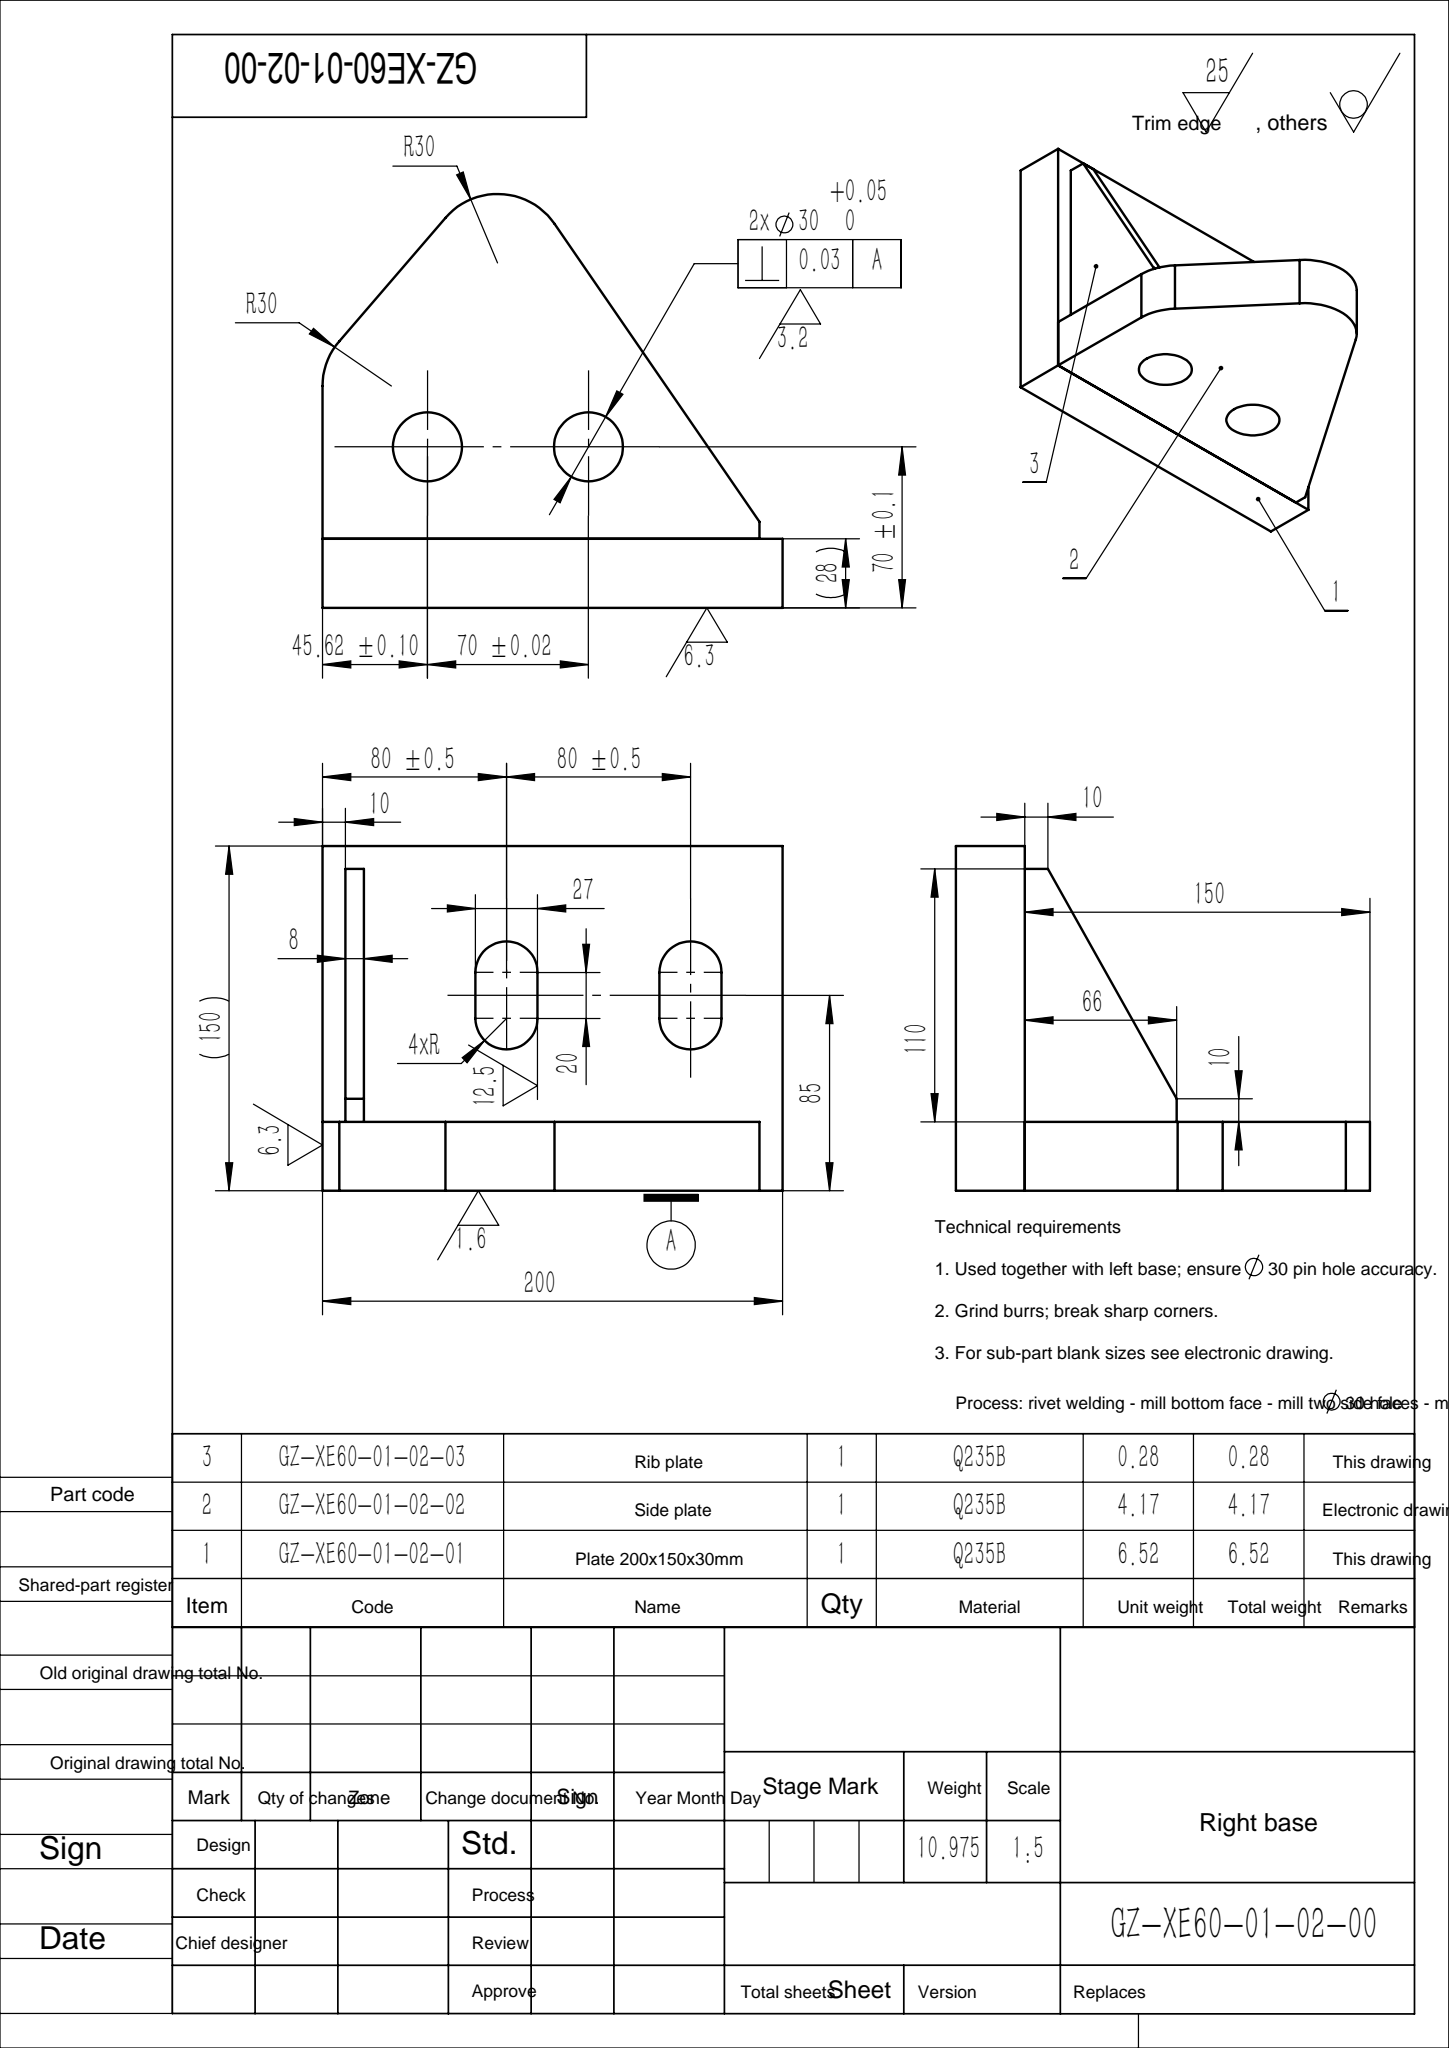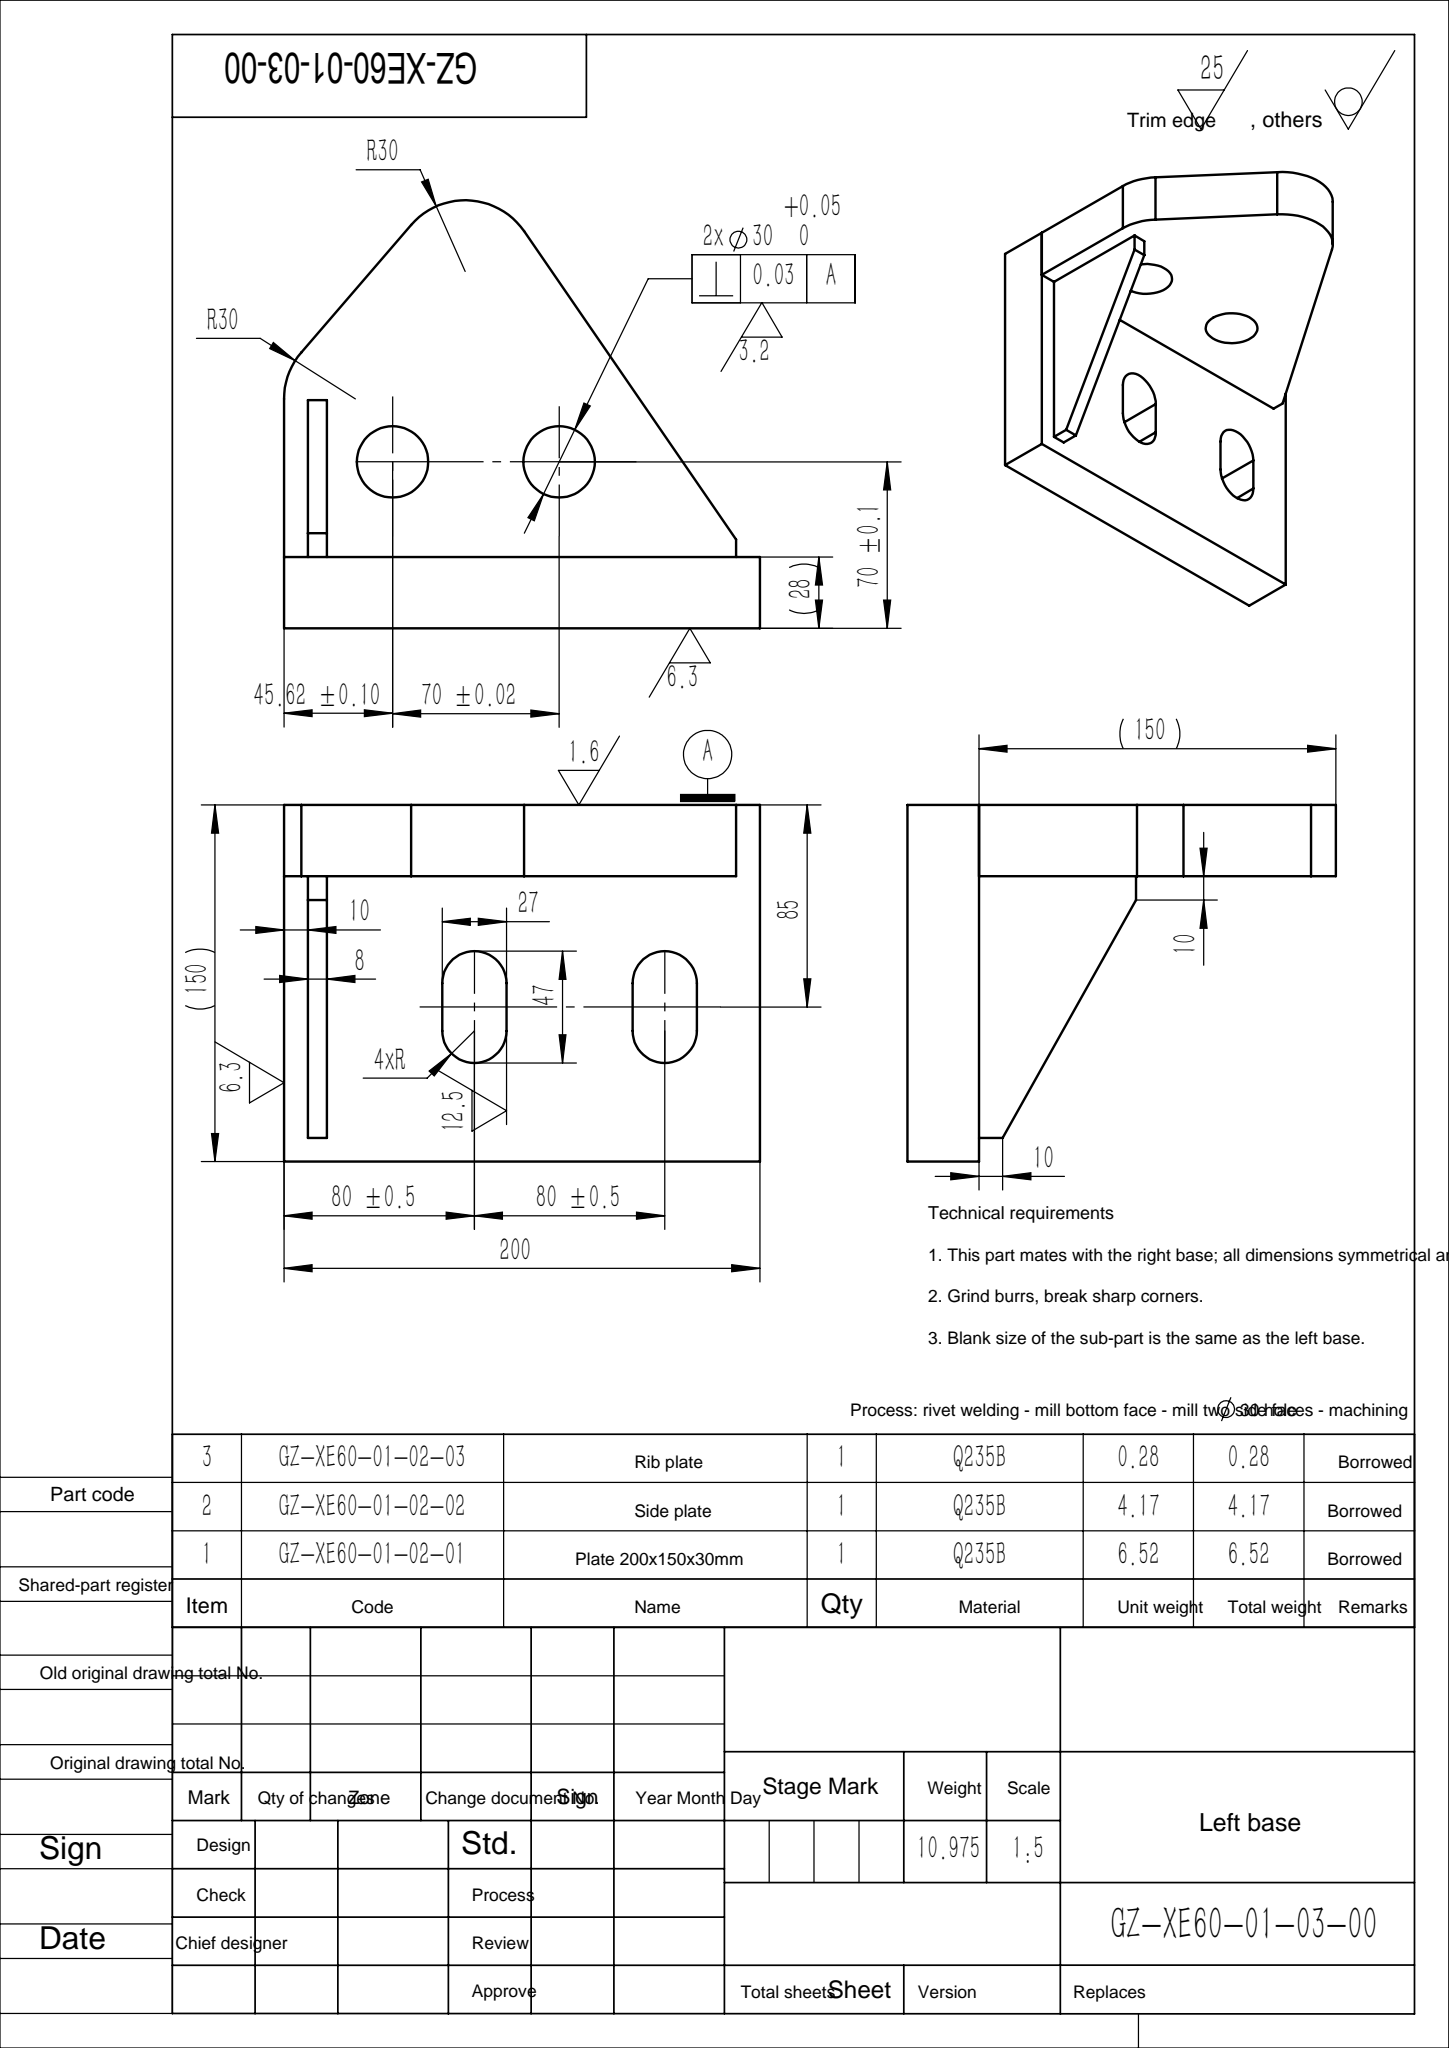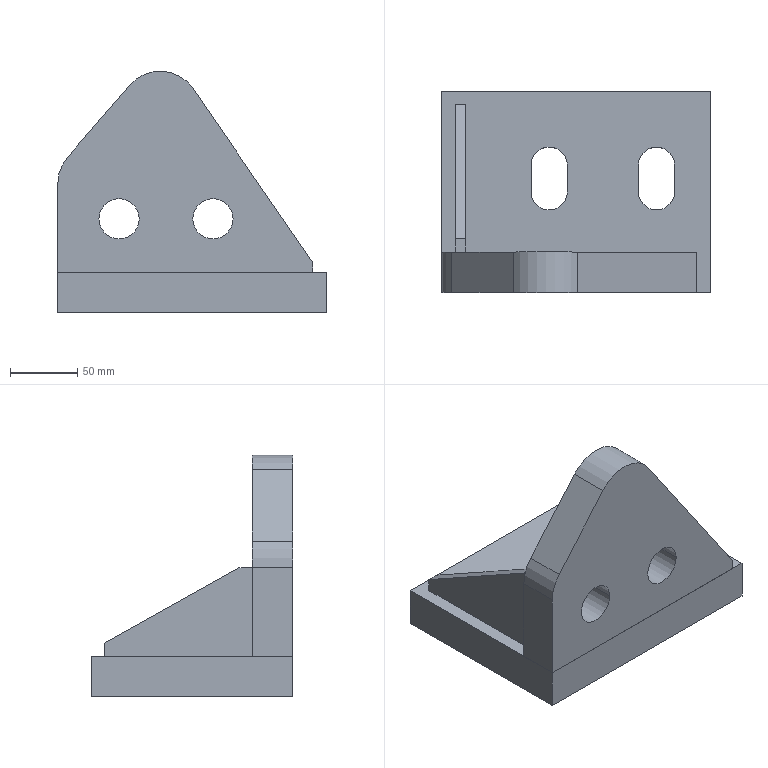Part | SolidWorks | 3 solids | 34 faces | box 200 x 150 x 180.029 mm | volume 1401678 mm3 | plane 24 | cylinder 10 | commonest cylinder face diameters 27 x4 30 x4 60 x2